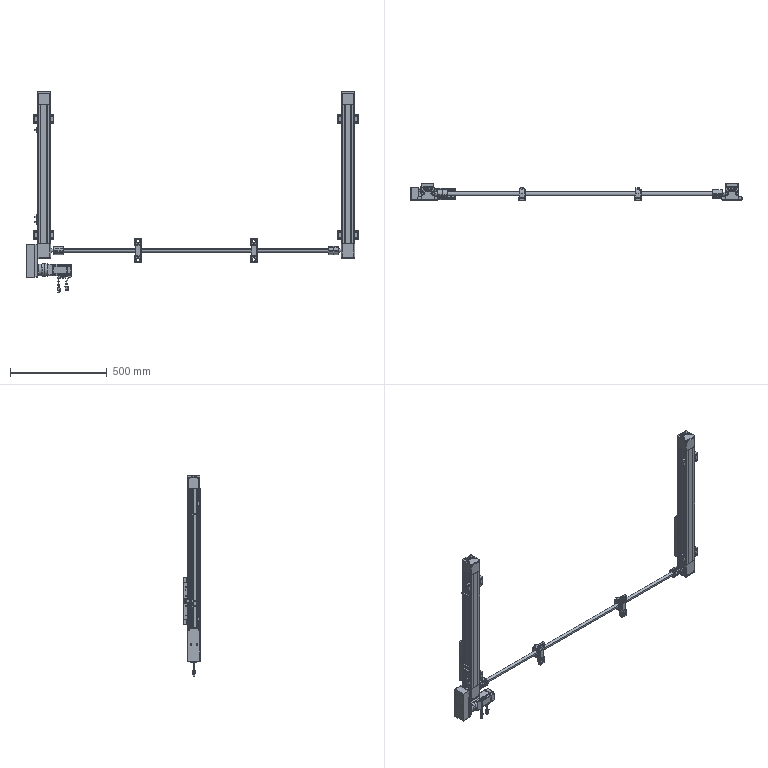Part | SolidWorks | 36 solids | 5002 faces | volume 9829860 mm3 | plane 2475 | cylinder 1458 | cone 754 | spline 221 | torus 68 | sphere 26 | commonest cylinder face diameters 6 x117 0.6 x107 1 x105 5.5 x104 5 x93 8 x81